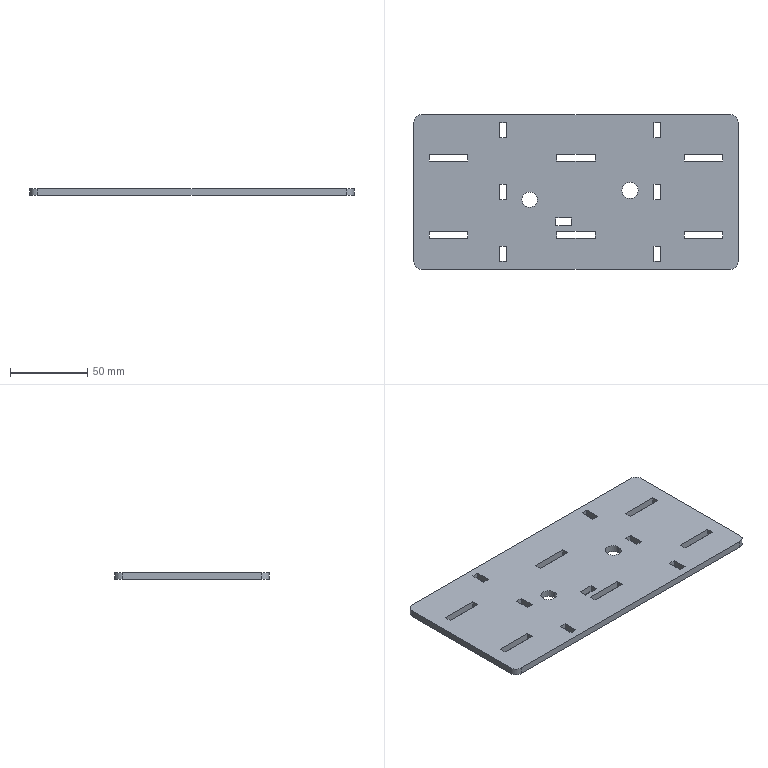Part | SolidWorks | features FlatPattern 1, SMBaseFlange 1, SheetMetal 1 | 1 solid | 66 faces | box 210 x 100 x 4.5 mm | volume 89183 mm3 | plane 58 | cylinder 8 | commonest cylinder face diameters 10 x6 10.5 x2